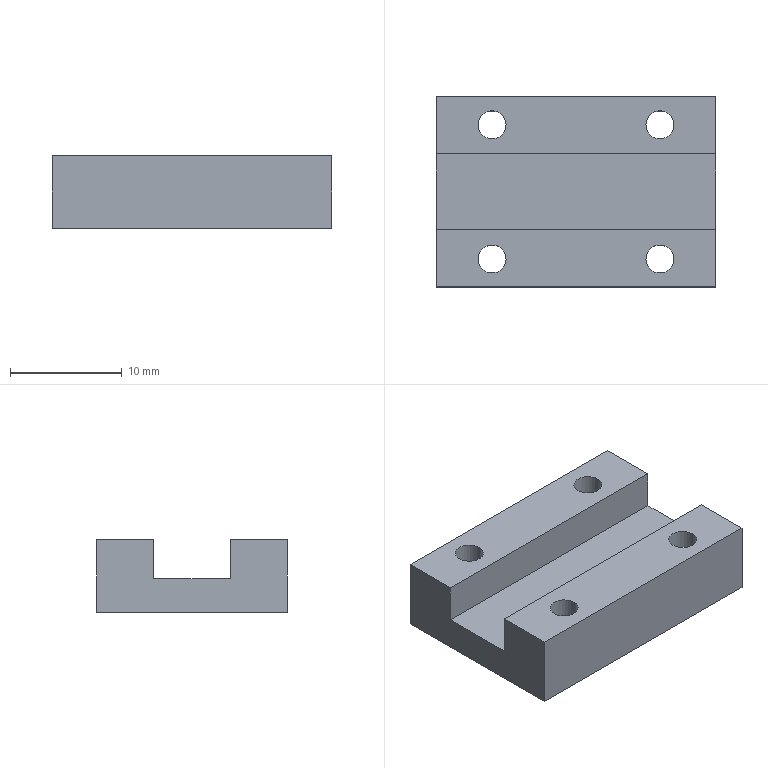Part | SolidWorks | features ICE 2, Extrusion 1 | 1 solid | 18 faces | box 25 x 17 x 6.5 mm | volume 2040 mm3 | plane 10 | cylinder 8 | commonest cylinder face diameters 2.5 x8
STEP:
#1=CARTESIAN_POINT('',(8.233,9.026,0.));
#2=VERTEX_POINT('',#1);
#3=CARTESIAN_POINT('',(5.733,9.026,0.));
#4=VERTEX_POINT('',#3);
#5=CARTESIAN_POINT('',(6.983,9.026,0.));
#6=DIRECTION('',(0.,0.,-1.));
#7=DIRECTION('',(1.,0.,0.));
#8=AXIS2_PLACEMENT_3D('',#5,#6,#7);
#9=CIRCLE('',#8,1.25);
#10=EDGE_CURVE('',#2,#4,#9,.T.);
#11=ORIENTED_EDGE('',*,*,#10,.T.);
#12=CARTESIAN_POINT('',(5.733,9.026,6.5));
#13=VERTEX_POINT('',#12);
#14=CARTESIAN_POINT('',(5.733,9.026,-0.001));
#15=DIRECTION('',(0.,0.,1.));
#16=VECTOR('',#15,1000.);
#17=LINE('',#14,#16);
#18=EDGE_CURVE('',#4,#13,#17,.T.);
#19=ORIENTED_EDGE('',*,*,#18,.T.);
#20=CARTESIAN_POINT('',(8.233,9.026,6.5));
#21=VERTEX_POINT('',#20);
#22=CARTESIAN_POINT('',(6.983,9.026,6.5));
#23=DIRECTION('',(0.,0.,1.));
#24=DIRECTION('',(1.,0.,0.));
#25=AXIS2_PLACEMENT_3D('',#22,#23,#24);
#26=CIRCLE('',#25,1.25);
#27=EDGE_CURVE('',#13,#21,#26,.T.);
#28=ORIENTED_EDGE('',*,*,#27,.T.);
#29=CARTESIAN_POINT('',(8.233,9.026,-0.001));
#30=DIRECTION('',(0.,0.,1.));
#31=VECTOR('',#30,1000.);
#32=LINE('',#29,#31);
#33=EDGE_CURVE('',#2,#21,#32,.T.);
#34=ORIENTED_EDGE('',*,*,#33,.F.);
#35=EDGE_LOOP('',(#11,#19,#28,#34));
#36=FACE_OUTER_BOUND('',#35,.T.);
#37=CARTESIAN_POINT('',(6.983,9.026,-0.001));
#38=DIRECTION('',(0.,0.,1.));
#39=DIRECTION('',(1.,0.,0.));
#40=AXIS2_PLACEMENT_3D('',#37,#38,#39);
#41=CYLINDRICAL_SURFACE('',#40,1.25);
#42=ADVANCED_FACE('',(#36),#41,.F.);
#43=CARTESIAN_POINT('',(-6.767,-2.974,0.));
#44=VERTEX_POINT('',#43);
#45=CARTESIAN_POINT('',(-9.267,-2.974,0.));
#46=VERTEX_POINT('',#45);
#47=CARTESIAN_POINT('',(-8.017,-2.974,0.));
#48=DIRECTION('',(0.,0.,-1.));
#49=DIRECTION('',(1.,0.,0.));
#50=AXIS2_PLACEMENT_3D('',#47,#48,#49);
#51=CIRCLE('',#50,1.25);
#52=EDGE_CURVE('',#44,#46,#51,.T.);
#53=ORIENTED_EDGE('',*,*,#52,.T.);
#54=CARTESIAN_POINT('',(-9.267,-2.974,6.5));
#55=VERTEX_POINT('',#54);
#56=CARTESIAN_POINT('',(-9.267,-2.974,-0.001));
#57=DIRECTION('',(0.,0.,1.));
#58=VECTOR('',#57,1000.);
#59=LINE('',#56,#58);
#60=EDGE_CURVE('',#46,#55,#59,.T.);
#61=ORIENTED_EDGE('',*,*,#60,.T.);
#62=CARTESIAN_POINT('',(-6.767,-2.974,6.5));
#63=VERTEX_POINT('',#62);
#64=CARTESIAN_POINT('',(-8.017,-2.974,6.5));
#65=DIRECTION('',(0.,0.,1.));
#66=DIRECTION('',(1.,0.,0.));
#67=AXIS2_PLACEMENT_3D('',#64,#65,#66);
#68=CIRCLE('',#67,1.25);
#69=EDGE_CURVE('',#55,#63,#68,.T.);
#70=ORIENTED_EDGE('',*,*,#69,.T.);
#71=CARTESIAN_POINT('',(-6.767,-2.974,-0.001));
#72=DIRECTION('',(0.,0.,1.));
#73=VECTOR('',#72,1000.);
#74=LINE('',#71,#73);
#75=EDGE_CURVE('',#44,#63,#74,.T.);
#76=ORIENTED_EDGE('',*,*,#75,.F.);
#77=EDGE_LOOP('',(#53,#61,#70,#76));
#78=FACE_OUTER_BOUND('',#77,.T.);
#79=CARTESIAN_POINT('',(-8.017,-2.974,-0.001));
#80=DIRECTION('',(0.,0.,1.));
#81=DIRECTION('',(1.,0.,0.));
#82=AXIS2_PLACEMENT_3D('',#79,#80,#81);
#83=CYLINDRICAL_SURFACE('',#82,1.25);
#84=ADVANCED_FACE('',(#78),#83,.F.);
#85=CARTESIAN_POINT('',(8.233,-2.974,0.));
#86=VERTEX_POINT('',#85);
#87=CARTESIAN_POINT('',(5.733,-2.974,0.));
#88=VERTEX_POINT('',#87);
#89=CARTESIAN_POINT('',(6.983,-2.974,0.));
#90=DIRECTION('',(0.,0.,-1.));
#91=DIRECTION('',(1.,0.,0.));
#92=AXIS2_PLACEMENT_3D('',#89,#90,#91);
#93=CIRCLE('',#92,1.25);
#94=EDGE_CURVE('',#86,#88,#93,.T.);
#95=ORIENTED_EDGE('',*,*,#94,.T.);
#96=CARTESIAN_POINT('',(5.733,-2.974,6.5));
#97=VERTEX_POINT('',#96);
#98=CARTESIAN_POINT('',(5.733,-2.974,-0.001));
#99=DIRECTION('',(0.,0.,1.));
#100=VECTOR('',#99,1000.);
#101=LINE('',#98,#100);
#102=EDGE_CURVE('',#88,#97,#101,.T.);
#103=ORIENTED_EDGE('',*,*,#102,.T.);
#104=CARTESIAN_POINT('',(8.233,-2.974,6.5));
#105=VERTEX_POINT('',#104);
#106=CARTESIAN_POINT('',(6.983,-2.974,6.5));
#107=DIRECTION('',(0.,0.,1.));
#108=DIRECTION('',(1.,0.,0.));
#109=AXIS2_PLACEMENT_3D('',#106,#107,#108);
#110=CIRCLE('',#109,1.25);
#111=EDGE_CURVE('',#97,#105,#110,.T.);
#112=ORIENTED_EDGE('',*,*,#111,.T.);
#113=CARTESIAN_POINT('',(8.233,-2.974,-0.001));
#114=DIRECTION('',(0.,0.,1.));
#115=VECTOR('',#114,1000.);
#116=LINE('',#113,#115);
#117=EDGE_CURVE('',#86,#105,#116,.T.);
#118=ORIENTED_EDGE('',*,*,#117,.F.);
#119=EDGE_LOOP('',(#95,#103,#112,#118));
#120=FACE_OUTER_BOUND('',#119,.T.);
#121=CARTESIAN_POINT('',(6.983,-2.974,-0.001));
#122=DIRECTION('',(0.,0.,1.));
#123=DIRECTION('',(1.,0.,0.));
#124=AXIS2_PLACEMENT_3D('',#121,#122,#123);
#125=CYLINDRICAL_SURFACE('',#124,1.25);
#126=ADVANCED_FACE('',(#120),#125,.F.);
#127=CARTESIAN_POINT('',(-6.767,9.026,0.));
#128=VERTEX_POINT('',#127);
#129=CARTESIAN_POINT('',(-9.267,9.026,0.));
#130=VERTEX_POINT('',#129);
#131=CARTESIAN_POINT('',(-8.017,9.026,0.));
#132=DIRECTION('',(0.,0.,-1.));
#133=DIRECTION('',(1.,0.,0.));
#134=AXIS2_PLACEMENT_3D('',#131,#132,#133);
#135=CIRCLE('',#134,1.25);
#136=EDGE_CURVE('',#128,#130,#135,.T.);
#137=ORIENTED_EDGE('',*,*,#136,.T.);
#138=CARTESIAN_POINT('',(-9.267,9.026,6.5));
#139=VERTEX_POINT('',#138);
#140=CARTESIAN_POINT('',(-9.267,9.026,-0.001));
#141=DIRECTION('',(0.,0.,1.));
#142=VECTOR('',#141,1000.);
#143=LINE('',#140,#142);
#144=EDGE_CURVE('',#130,#139,#143,.T.);
#145=ORIENTED_EDGE('',*,*,#144,.T.);
#146=CARTESIAN_POINT('',(-6.767,9.026,6.5));
#147=VERTEX_POINT('',#146);
#148=CARTESIAN_POINT('',(-8.017,9.026,6.5));
#149=DIRECTION('',(0.,0.,1.));
#150=DIRECTION('',(1.,0.,0.));
#151=AXIS2_PLACEMENT_3D('',#148,#149,#150);
#152=CIRCLE('',#151,1.25);
#153=EDGE_CURVE('',#139,#147,#152,.T.);
#154=ORIENTED_EDGE('',*,*,#153,.T.);
#155=CARTESIAN_POINT('',(-6.767,9.026,-0.001));
#156=DIRECTION('',(0.,0.,1.));
#157=VECTOR('',#156,1000.);
#158=LINE('',#155,#157);
#159=EDGE_CURVE('',#128,#147,#158,.T.);
#160=ORIENTED_EDGE('',*,*,#159,.F.);
#161=EDGE_LOOP('',(#137,#145,#154,#160));
#162=FACE_OUTER_BOUND('',#161,.T.);
#163=CARTESIAN_POINT('',(-8.017,9.026,-0.001));
#164=DIRECTION('',(0.,0.,1.));
#165=DIRECTION('',(1.,0.,0.));
#166=AXIS2_PLACEMENT_3D('',#163,#164,#165);
#167=CYLINDRICAL_SURFACE('',#166,1.25);
#168=ADVANCED_FACE('',(#162),#167,.F.);
#169=CARTESIAN_POINT('',(6.983,9.026,6.5));
#170=DIRECTION('',(0.,0.,1.));
#171=DIRECTION('',(1.,0.,0.));
#172=AXIS2_PLACEMENT_3D('',#169,#170,#171);
#173=CIRCLE('',#172,1.25);
#174=EDGE_CURVE('',#21,#13,#173,.T.);
#175=ORIENTED_EDGE('',*,*,#174,.F.);
#176=ORIENTED_EDGE('',*,*,#27,.F.);
#177=EDGE_LOOP('',(#175,#176));
#178=FACE_BOUND('',#177,.T.);
#179=CARTESIAN_POINT('',(-8.017,9.026,6.5));
#180=DIRECTION('',(0.,0.,1.));
#181=DIRECTION('',(1.,0.,0.));
#182=AXIS2_PLACEMENT_3D('',#179,#180,#181);
#183=CIRCLE('',#182,1.25);
#184=EDGE_CURVE('',#147,#139,#183,.T.);
#185=ORIENTED_EDGE('',*,*,#184,.F.);
#186=ORIENTED_EDGE('',*,*,#153,.F.);
#187=EDGE_LOOP('',(#185,#186));
#188=FACE_BOUND('',#187,.T.);
#189=CARTESIAN_POINT('',(-13.017,6.426,6.5));
#190=VERTEX_POINT('',#189);
#191=CARTESIAN_POINT('',(11.983,6.426,6.5));
#192=VERTEX_POINT('',#191);
#193=CARTESIAN_POINT('',(-13.018,6.426,6.5));
#194=DIRECTION('',(1.,0.,0.));
#195=VECTOR('',#194,1000.);
#196=LINE('',#193,#195);
#197=EDGE_CURVE('',#190,#192,#196,.T.);
#198=ORIENTED_EDGE('',*,*,#197,.T.);
#199=CARTESIAN_POINT('',(11.983,11.526,6.5));
#200=VERTEX_POINT('',#199);
#201=CARTESIAN_POINT('',(11.983,11.526,6.5));
#202=DIRECTION('',(0.,1.,0.));
#203=VECTOR('',#202,1000.);
#204=LINE('',#201,#203);
#205=EDGE_CURVE('',#192,#200,#204,.T.);
#206=ORIENTED_EDGE('',*,*,#205,.T.);
#207=CARTESIAN_POINT('',(-13.017,11.526,6.5));
#208=VERTEX_POINT('',#207);
#209=CARTESIAN_POINT('',(-13.017,11.526,6.5));
#210=DIRECTION('',(-1.,0.,0.));
#211=VECTOR('',#210,1000.);
#212=LINE('',#209,#211);
#213=EDGE_CURVE('',#200,#208,#212,.T.);
#214=ORIENTED_EDGE('',*,*,#213,.T.);
#215=CARTESIAN_POINT('',(-13.017,11.526,6.5));
#216=DIRECTION('',(0.,-1.,0.));
#217=VECTOR('',#216,1000.);
#218=LINE('',#215,#217);
#219=EDGE_CURVE('',#208,#190,#218,.T.);
#220=ORIENTED_EDGE('',*,*,#219,.T.);
#221=EDGE_LOOP('',(#198,#206,#214,#220));
#222=FACE_OUTER_BOUND('',#221,.T.);
#223=CARTESIAN_POINT('',(0.,0.,6.5));
#224=DIRECTION('',(0.,0.,1.));
#225=DIRECTION('',(1.,0.,0.));
#226=AXIS2_PLACEMENT_3D('',#223,#224,#225);
#227=PLANE('',#226);
#228=ADVANCED_FACE('',(#178,#188,#222),#227,.T.);
#229=CARTESIAN_POINT('',(-13.017,6.426,3.));
#230=VERTEX_POINT('',#229);
#231=CARTESIAN_POINT('',(-13.017,-0.3739,3.));
#232=VERTEX_POINT('',#231);
#233=CARTESIAN_POINT('',(-13.017,-0.3739,3.));
#234=DIRECTION('',(0.,-1.,0.));
#235=VECTOR('',#234,1000.);
#236=LINE('',#233,#235);
#237=EDGE_CURVE('',#230,#232,#236,.T.);
#238=ORIENTED_EDGE('',*,*,#237,.F.);
#239=CARTESIAN_POINT('',(-13.017,6.426,6.5));
#240=DIRECTION('',(0.,0.,-1.));
#241=VECTOR('',#240,1000.);
#242=LINE('',#239,#241);
#243=EDGE_CURVE('',#190,#230,#242,.T.);
#244=ORIENTED_EDGE('',*,*,#243,.F.);
#245=ORIENTED_EDGE('',*,*,#219,.F.);
#246=CARTESIAN_POINT('',(-13.017,11.526,0.));
#247=VERTEX_POINT('',#246);
#248=CARTESIAN_POINT('',(-13.017,11.526,6.5));
#249=DIRECTION('',(0.,0.,-1.));
#250=VECTOR('',#249,1000.);
#251=LINE('',#248,#250);
#252=EDGE_CURVE('',#208,#247,#251,.T.);
#253=ORIENTED_EDGE('',*,*,#252,.T.);
#254=CARTESIAN_POINT('',(-13.017,-5.474,0.));
#255=VERTEX_POINT('',#254);
#256=CARTESIAN_POINT('',(-13.017,11.526,0.));
#257=DIRECTION('',(0.,-1.,0.));
#258=VECTOR('',#257,1000.);
#259=LINE('',#256,#258);
#260=EDGE_CURVE('',#247,#255,#259,.T.);
#261=ORIENTED_EDGE('',*,*,#260,.T.);
#262=CARTESIAN_POINT('',(-13.017,-5.474,6.5));
#263=VERTEX_POINT('',#262);
#264=CARTESIAN_POINT('',(-13.017,-5.474,6.5));
#265=DIRECTION('',(0.,0.,-1.));
#266=VECTOR('',#265,1000.);
#267=LINE('',#264,#266);
#268=EDGE_CURVE('',#263,#255,#267,.T.);
#269=ORIENTED_EDGE('',*,*,#268,.F.);
#270=CARTESIAN_POINT('',(-13.017,-0.3739,6.5));
#271=VERTEX_POINT('',#270);
#272=CARTESIAN_POINT('',(-13.017,11.526,6.5));
#273=DIRECTION('',(0.,-1.,0.));
#274=VECTOR('',#273,1000.);
#275=LINE('',#272,#274);
#276=EDGE_CURVE('',#271,#263,#275,.T.);
#277=ORIENTED_EDGE('',*,*,#276,.F.);
#278=CARTESIAN_POINT('',(-13.017,-0.3739,6.5));
#279=DIRECTION('',(0.,0.,1.));
#280=VECTOR('',#279,1000.);
#281=LINE('',#278,#280);
#282=EDGE_CURVE('',#232,#271,#281,.T.);
#283=ORIENTED_EDGE('',*,*,#282,.F.);
#284=EDGE_LOOP('',(#238,#244,#245,#253,#261,#269,#277,#283));
#285=FACE_OUTER_BOUND('',#284,.T.);
#286=CARTESIAN_POINT('',(-13.017,11.526,6.5));
#287=DIRECTION('',(1.,0.,0.));
#288=DIRECTION('',(0.,0.,-1.));
#289=AXIS2_PLACEMENT_3D('',#286,#287,#288);
#290=PLANE('',#289);
#291=ADVANCED_FACE('',(#285),#290,.F.);
#292=CARTESIAN_POINT('',(11.983,-5.474,0.));
#293=VERTEX_POINT('',#292);
#294=CARTESIAN_POINT('',(-13.017,-5.474,0.));
#295=DIRECTION('',(1.,0.,0.));
#296=VECTOR('',#295,1000.);
#297=LINE('',#294,#296);
#298=EDGE_CURVE('',#255,#293,#297,.T.);
#299=ORIENTED_EDGE('',*,*,#298,.T.);
#300=CARTESIAN_POINT('',(11.983,-5.474,6.5));
#301=VERTEX_POINT('',#300);
#302=CARTESIAN_POINT('',(11.983,-5.474,6.5));
#303=DIRECTION('',(0.,0.,-1.));
#304=VECTOR('',#303,1000.);
#305=LINE('',#302,#304);
#306=EDGE_CURVE('',#301,#293,#305,.T.);
#307=ORIENTED_EDGE('',*,*,#306,.F.);
#308=CARTESIAN_POINT('',(-13.017,-5.474,6.5));
#309=DIRECTION('',(1.,0.,0.));
#310=VECTOR('',#309,1000.);
#311=LINE('',#308,#310);
#312=EDGE_CURVE('',#263,#301,#311,.T.);
#313=ORIENTED_EDGE('',*,*,#312,.F.);
#314=ORIENTED_EDGE('',*,*,#268,.T.);
#315=EDGE_LOOP('',(#299,#307,#313,#314));
#316=FACE_OUTER_BOUND('',#315,.T.);
#317=CARTESIAN_POINT('',(-13.017,-5.474,6.5));
#318=DIRECTION('',(0.,1.,0.));
#319=DIRECTION('',(0.,0.,1.));
#320=AXIS2_PLACEMENT_3D('',#317,#318,#319);
#321=PLANE('',#320);
#322=ADVANCED_FACE('',(#316),#321,.F.);
#323=ORIENTED_EDGE('',*,*,#205,.F.);
#324=CARTESIAN_POINT('',(11.983,6.426,3.));
#325=VERTEX_POINT('',#324);
#326=CARTESIAN_POINT('',(11.983,6.426,6.5));
#327=DIRECTION('',(0.,0.,1.));
#328=VECTOR('',#327,1000.);
#329=LINE('',#326,#328);
#330=EDGE_CURVE('',#325,#192,#329,.T.);
#331=ORIENTED_EDGE('',*,*,#330,.F.);
#332=CARTESIAN_POINT('',(11.983,-0.3739,3.));
#333=VERTEX_POINT('',#332);
#334=CARTESIAN_POINT('',(11.983,-0.3739,3.));
#335=DIRECTION('',(0.,1.,0.));
#336=VECTOR('',#335,1000.);
#337=LINE('',#334,#336);
#338=EDGE_CURVE('',#333,#325,#337,.T.);
#339=ORIENTED_EDGE('',*,*,#338,.F.);
#340=CARTESIAN_POINT('',(11.983,-0.3739,6.5));
#341=VERTEX_POINT('',#340);
#342=CARTESIAN_POINT('',(11.983,-0.3739,6.5));
#343=DIRECTION('',(0.,0.,-1.));
#344=VECTOR('',#343,1000.);
#345=LINE('',#342,#344);
#346=EDGE_CURVE('',#341,#333,#345,.T.);
#347=ORIENTED_EDGE('',*,*,#346,.F.);
#348=CARTESIAN_POINT('',(11.983,11.526,6.5));
#349=DIRECTION('',(0.,1.,0.));
#350=VECTOR('',#349,1000.);
#351=LINE('',#348,#350);
#352=EDGE_CURVE('',#301,#341,#351,.T.);
#353=ORIENTED_EDGE('',*,*,#352,.F.);
#354=ORIENTED_EDGE('',*,*,#306,.T.);
#355=CARTESIAN_POINT('',(11.983,11.526,0.));
#356=VERTEX_POINT('',#355);
#357=CARTESIAN_POINT('',(11.983,11.526,0.));
#358=DIRECTION('',(0.,1.,0.));
#359=VECTOR('',#358,1000.);
#360=LINE('',#357,#359);
#361=EDGE_CURVE('',#293,#356,#360,.T.);
#362=ORIENTED_EDGE('',*,*,#361,.T.);
#363=CARTESIAN_POINT('',(11.983,11.526,6.5));
#364=DIRECTION('',(0.,0.,-1.));
#365=VECTOR('',#364,1000.);
#366=LINE('',#363,#365);
#367=EDGE_CURVE('',#200,#356,#366,.T.);
#368=ORIENTED_EDGE('',*,*,#367,.F.);
#369=EDGE_LOOP('',(#323,#331,#339,#347,#353,#354,#362,#368));
#370=FACE_OUTER_BOUND('',#369,.T.);
#371=CARTESIAN_POINT('',(11.983,11.526,6.5));
#372=DIRECTION('',(-1.,0.,0.));
#373=DIRECTION('',(0.,-1.,0.));
#374=AXIS2_PLACEMENT_3D('',#371,#372,#373);
#375=PLANE('',#374);
#376=ADVANCED_FACE('',(#370),#375,.F.);
#377=CARTESIAN_POINT('',(-13.017,11.526,0.));
#378=DIRECTION('',(-1.,0.,0.));
#379=VECTOR('',#378,1000.);
#380=LINE('',#377,#379);
#381=EDGE_CURVE('',#356,#247,#380,.T.);
#382=ORIENTED_EDGE('',*,*,#381,.T.);
#383=ORIENTED_EDGE('',*,*,#252,.F.);
#384=ORIENTED_EDGE('',*,*,#213,.F.);
#385=ORIENTED_EDGE('',*,*,#367,.T.);
#386=EDGE_LOOP('',(#382,#383,#384,#385));
#387=FACE_OUTER_BOUND('',#386,.T.);
#388=CARTESIAN_POINT('',(-13.017,11.526,6.5));
#389=DIRECTION('',(0.,-1.,0.));
#390=DIRECTION('',(0.,0.,-1.));
#391=AXIS2_PLACEMENT_3D('',#388,#389,#390);
#392=PLANE('',#391);
#393=ADVANCED_FACE('',(#387),#392,.F.);
#394=CARTESIAN_POINT('',(-8.017,-2.974,6.5));
#395=DIRECTION('',(0.,0.,1.));
#396=DIRECTION('',(1.,0.,0.));
#397=AXIS2_PLACEMENT_3D('',#394,#395,#396);
#398=CIRCLE('',#397,1.25);
#399=EDGE_CURVE('',#63,#55,#398,.T.);
#400=ORIENTED_EDGE('',*,*,#399,.F.);
#401=ORIENTED_EDGE('',*,*,#69,.F.);
#402=EDGE_LOOP('',(#400,#401));
#403=FACE_BOUND('',#402,.T.);
#404=CARTESIAN_POINT('',(6.983,-2.974,6.5));
#405=DIRECTION('',(0.,0.,1.));
#406=DIRECTION('',(1.,0.,0.));
#407=AXIS2_PLACEMENT_3D('',#404,#405,#406);
#408=CIRCLE('',#407,1.25);
#409=EDGE_CURVE('',#105,#97,#408,.T.);
#410=ORIENTED_EDGE('',*,*,#409,.F.);
#411=ORIENTED_EDGE('',*,*,#111,.F.);
#412=EDGE_LOOP('',(#410,#411));
#413=FACE_BOUND('',#412,.T.);
#414=CARTESIAN_POINT('',(-13.018,-0.3739,6.5));
#415=DIRECTION('',(1.,0.,0.));
#416=VECTOR('',#415,1000.);
#417=LINE('',#414,#416);
#418=EDGE_CURVE('',#271,#341,#417,.T.);
#419=ORIENTED_EDGE('',*,*,#418,.F.);
#420=ORIENTED_EDGE('',*,*,#276,.T.);
#421=ORIENTED_EDGE('',*,*,#312,.T.);
#422=ORIENTED_EDGE('',*,*,#352,.T.);
#423=EDGE_LOOP('',(#419,#420,#421,#422));
#424=FACE_OUTER_BOUND('',#423,.T.);
#425=CARTESIAN_POINT('',(0.,0.,6.5));
#426=DIRECTION('',(0.,0.,1.));
#427=DIRECTION('',(1.,0.,0.));
#428=AXIS2_PLACEMENT_3D('',#425,#426,#427);
#429=PLANE('',#428);
#430=ADVANCED_FACE('',(#403,#413,#424),#429,.T.);
#431=ORIENTED_EDGE('',*,*,#10,.F.);
#432=CARTESIAN_POINT('',(6.983,9.026,0.));
#433=DIRECTION('',(0.,0.,-1.));
#434=DIRECTION('',(1.,0.,0.));
#435=AXIS2_PLACEMENT_3D('',#432,#433,#434);
#436=CIRCLE('',#435,1.25);
#437=EDGE_CURVE('',#4,#2,#436,.T.);
#438=ORIENTED_EDGE('',*,*,#437,.F.);
#439=EDGE_LOOP('',(#431,#438));
#440=FACE_BOUND('',#439,.T.);
#441=ORIENTED_EDGE('',*,*,#52,.F.);
#442=CARTESIAN_POINT('',(-8.017,-2.974,0.));
#443=DIRECTION('',(0.,0.,-1.));
#444=DIRECTION('',(1.,0.,0.));
#445=AXIS2_PLACEMENT_3D('',#442,#443,#444);
#446=CIRCLE('',#445,1.25);
#447=EDGE_CURVE('',#46,#44,#446,.T.);
#448=ORIENTED_EDGE('',*,*,#447,.F.);
#449=EDGE_LOOP('',(#441,#448));
#450=FACE_BOUND('',#449,.T.);
#451=ORIENTED_EDGE('',*,*,#94,.F.);
#452=CARTESIAN_POINT('',(6.983,-2.974,0.));
#453=DIRECTION('',(0.,0.,-1.));
#454=DIRECTION('',(1.,0.,0.));
#455=AXIS2_PLACEMENT_3D('',#452,#453,#454);
#456=CIRCLE('',#455,1.25);
#457=EDGE_CURVE('',#88,#86,#456,.T.);
#458=ORIENTED_EDGE('',*,*,#457,.F.);
#459=EDGE_LOOP('',(#451,#458));
#460=FACE_BOUND('',#459,.T.);
#461=ORIENTED_EDGE('',*,*,#136,.F.);
#462=CARTESIAN_POINT('',(-8.017,9.026,0.));
#463=DIRECTION('',(0.,0.,-1.));
#464=DIRECTION('',(1.,0.,0.));
#465=AXIS2_PLACEMENT_3D('',#462,#463,#464);
#466=CIRCLE('',#465,1.25);
#467=EDGE_CURVE('',#130,#128,#466,.T.);
#468=ORIENTED_EDGE('',*,*,#467,.F.);
#469=EDGE_LOOP('',(#461,#468));
#470=FACE_BOUND('',#469,.T.);
#471=ORIENTED_EDGE('',*,*,#260,.F.);
#472=ORIENTED_EDGE('',*,*,#381,.F.);
#473=ORIENTED_EDGE('',*,*,#361,.F.);
#474=ORIENTED_EDGE('',*,*,#298,.F.);
#475=EDGE_LOOP('',(#471,#472,#473,#474));
#476=FACE_OUTER_BOUND('',#475,.T.);
#477=CARTESIAN_POINT('',(0.,0.,0.));
#478=DIRECTION('',(0.,0.,1.));
#479=DIRECTION('',(1.,0.,0.));
#480=AXIS2_PLACEMENT_3D('',#477,#478,#479);
#481=PLANE('',#480);
#482=ADVANCED_FACE('',(#440,#450,#460,#470,#476),#481,.F.);
#483=ORIENTED_EDGE('',*,*,#243,.T.);
#484=CARTESIAN_POINT('',(-13.018,6.426,3.));
#485=DIRECTION('',(1.,0.,0.));
#486=VECTOR('',#485,1000.);
#487=LINE('',#484,#486);
#488=EDGE_CURVE('',#230,#325,#487,.T.);
#489=ORIENTED_EDGE('',*,*,#488,.T.);
#490=ORIENTED_EDGE('',*,*,#330,.T.);
#491=ORIENTED_EDGE('',*,*,#197,.F.);
#492=EDGE_LOOP('',(#483,#489,#490,#491));
#493=FACE_OUTER_BOUND('',#492,.T.);
#494=CARTESIAN_POINT('',(-13.018,6.426,6.5));
#495=DIRECTION('',(0.,1.,0.));
#496=DIRECTION('',(-1.,0.,0.));
#497=AXIS2_PLACEMENT_3D('',#494,#495,#496);
#498=PLANE('',#497);
#499=ADVANCED_FACE('',(#493),#498,.F.);
#500=ORIENTED_EDGE('',*,*,#237,.T.);
#501=CARTESIAN_POINT('',(-13.018,-0.3739,3.));
#502=DIRECTION('',(1.,0.,0.));
#503=VECTOR('',#502,1000.);
#504=LINE('',#501,#503);
#505=EDGE_CURVE('',#232,#333,#504,.T.);
#506=ORIENTED_EDGE('',*,*,#505,.T.);
#507=ORIENTED_EDGE('',*,*,#338,.T.);
#508=ORIENTED_EDGE('',*,*,#488,.F.);
#509=EDGE_LOOP('',(#500,#506,#507,#508));
#510=FACE_OUTER_BOUND('',#509,.T.);
#511=CARTESIAN_POINT('',(-13.018,-0.3739,3.));
#512=DIRECTION('',(0.,0.,-1.));
#513=DIRECTION('',(-1.,0.,0.));
#514=AXIS2_PLACEMENT_3D('',#511,#512,#513);
#515=PLANE('',#514);
#516=ADVANCED_FACE('',(#510),#515,.F.);
#517=ORIENTED_EDGE('',*,*,#282,.T.);
#518=ORIENTED_EDGE('',*,*,#418,.T.);
#519=ORIENTED_EDGE('',*,*,#346,.T.);
#520=ORIENTED_EDGE('',*,*,#505,.F.);
#521=EDGE_LOOP('',(#517,#518,#519,#520));
#522=FACE_OUTER_BOUND('',#521,.T.);
#523=CARTESIAN_POINT('',(-13.018,-0.3739,6.5));
#524=DIRECTION('',(0.,-1.,0.));
#525=DIRECTION('',(1.,0.,0.));
#526=AXIS2_PLACEMENT_3D('',#523,#524,#525);
#527=PLANE('',#526);
#528=ADVANCED_FACE('',(#522),#527,.F.);
#529=ORIENTED_EDGE('',*,*,#144,.F.);
#530=ORIENTED_EDGE('',*,*,#467,.T.);
#531=ORIENTED_EDGE('',*,*,#159,.T.);
#532=ORIENTED_EDGE('',*,*,#184,.T.);
#533=EDGE_LOOP('',(#529,#530,#531,#532));
#534=FACE_OUTER_BOUND('',#533,.T.);
#535=CARTESIAN_POINT('',(-8.017,9.026,-0.001));
#536=DIRECTION('',(0.,0.,1.));
#537=DIRECTION('',(1.,0.,0.));
#538=AXIS2_PLACEMENT_3D('',#535,#536,#537);
#539=CYLINDRICAL_SURFACE('',#538,1.25);
#540=ADVANCED_FACE('',(#534),#539,.F.);
#541=ORIENTED_EDGE('',*,*,#102,.F.);
#542=ORIENTED_EDGE('',*,*,#457,.T.);
#543=ORIENTED_EDGE('',*,*,#117,.T.);
#544=ORIENTED_EDGE('',*,*,#409,.T.);
#545=EDGE_LOOP('',(#541,#542,#543,#544));
#546=FACE_OUTER_BOUND('',#545,.T.);
#547=CARTESIAN_POINT('',(6.983,-2.974,-0.001));
#548=DIRECTION('',(0.,0.,1.));
#549=DIRECTION('',(1.,0.,0.));
#550=AXIS2_PLACEMENT_3D('',#547,#548,#549);
#551=CYLINDRICAL_SURFACE('',#550,1.25);
#552=ADVANCED_FACE('',(#546),#551,.F.);
#553=ORIENTED_EDGE('',*,*,#60,.F.);
#554=ORIENTED_EDGE('',*,*,#447,.T.);
#555=ORIENTED_EDGE('',*,*,#75,.T.);
#556=ORIENTED_EDGE('',*,*,#399,.T.);
#557=EDGE_LOOP('',(#553,#554,#555,#556));
#558=FACE_OUTER_BOUND('',#557,.T.);
#559=CARTESIAN_POINT('',(-8.017,-2.974,-0.001));
#560=DIRECTION('',(0.,0.,1.));
#561=DIRECTION('',(1.,0.,0.));
#562=AXIS2_PLACEMENT_3D('',#559,#560,#561);
#563=CYLINDRICAL_SURFACE('',#562,1.25);
#564=ADVANCED_FACE('',(#558),#563,.F.);
#565=ORIENTED_EDGE('',*,*,#18,.F.);
#566=ORIENTED_EDGE('',*,*,#437,.T.);
#567=ORIENTED_EDGE('',*,*,#33,.T.);
#568=ORIENTED_EDGE('',*,*,#174,.T.);
#569=EDGE_LOOP('',(#565,#566,#567,#568));
#570=FACE_OUTER_BOUND('',#569,.T.);
#571=CARTESIAN_POINT('',(6.983,9.026,-0.001));
#572=DIRECTION('',(0.,0.,1.));
#573=DIRECTION('',(1.,0.,0.));
#574=AXIS2_PLACEMENT_3D('',#571,#572,#573);
#575=CYLINDRICAL_SURFACE('',#574,1.25);
#576=ADVANCED_FACE('',(#570),#575,.F.);
#577=CLOSED_SHELL('',(#42,#84,#126,#168,#228,#291,#322,#376,#393,#430,#482,#499,#516,#528,#540,#552,#564,#576));
#578=MANIFOLD_SOLID_BREP('',#577);
#579=CARTESIAN_POINT('',(0.,0.,0.));
#580=DIRECTION('',(0.,0.,1.));
#581=DIRECTION('',(1.,0.,0.));
#582=AXIS2_PLACEMENT_3D('',#579,#580,#581);
#583=(LENGTH_UNIT()NAMED_UNIT(*)SI_UNIT(.MILLI.,.METRE.));
#584=UNCERTAINTY_MEASURE_WITH_UNIT(LENGTH_MEASURE(0.00001),#583,'','');
#585=(NAMED_UNIT(*)PLANE_ANGLE_UNIT()SI_UNIT($,.RADIAN.));
#586=(NAMED_UNIT(*)SI_UNIT($,.STERADIAN.)SOLID_ANGLE_UNIT());
#587=(GEOMETRIC_REPRESENTATION_CONTEXT(3)GLOBAL_UNCERTAINTY_ASSIGNED_CONTEXT((#584))GLOBAL_UNIT_ASSIGNED_CONTEXT((#583,#585,#586))REPRESENTATION_CONTEXT('',''));
#588=ADVANCED_BREP_SHAPE_REPRESENTATION('',(#578,#582),#587);